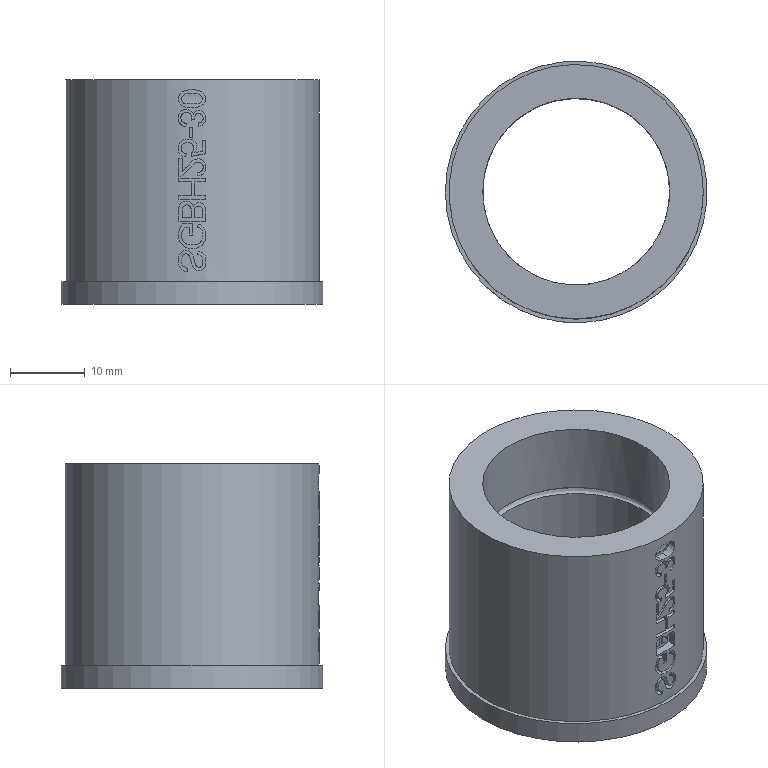Part | NX | features MI_SGBH_0847 2 | 1 solid | 144 faces | box 35 x 35 x 30 mm | volume 12569 mm3 | plane 77 | cylinder 65 | spline 2 | commonest cylinder face diameters 31.8 x9 25 x3 32 x3 2.113 x2 0.999 x1 1.035 x1